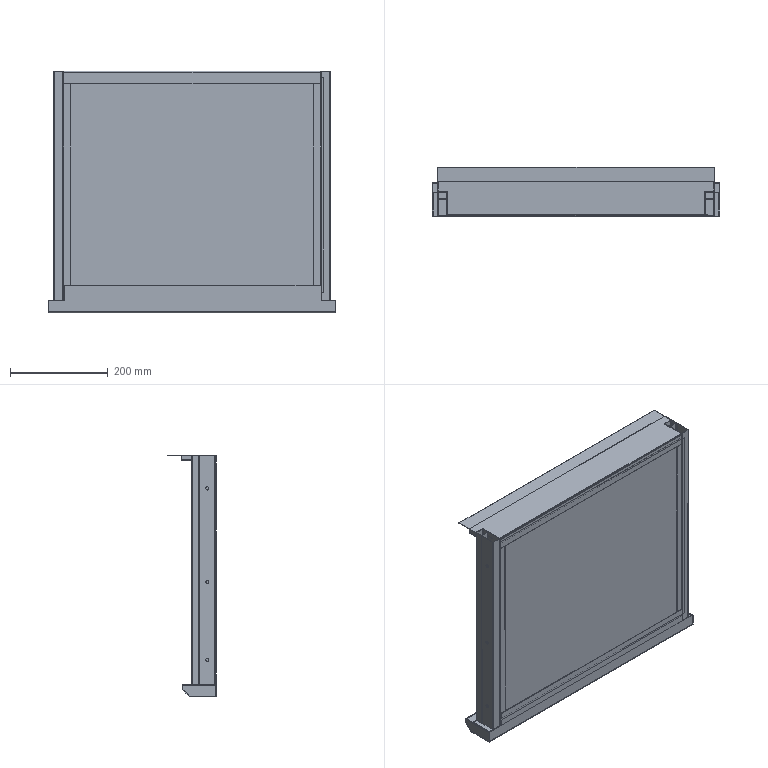Part | SolidWorks | features MirrorCompFeat 3, ReferencePattern 3, AEMSimFeature 1 | 11 solids | 566 faces | box 590 x 100 x 495 mm | volume 1096405 mm3 | plane 370 | cylinder 192 | spline 4 | commonest cylinder face diameters 2 x81 4 x47 1.686 x36 6.5 x12 2.4 x8 6 x4